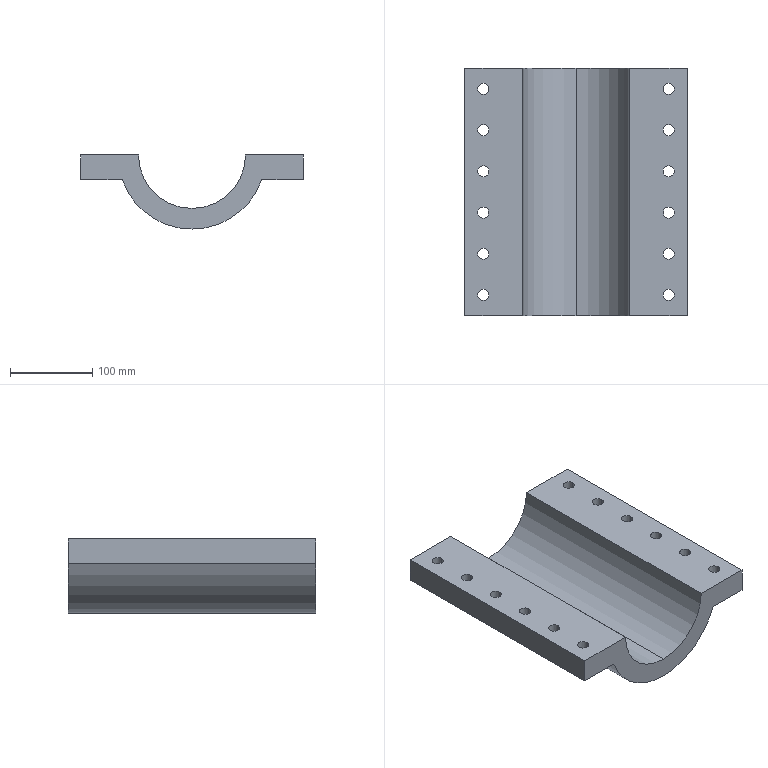Part | SolidWorks | features BaseBody 1 | 1 solid | 72 faces | box 270 x 300 x 90 mm | volume 2586327 mm3 | cylinder 52 | plane 20 | commonest cylinder face diameters 13.5 x24 23.78 x24 130 x2 180 x2